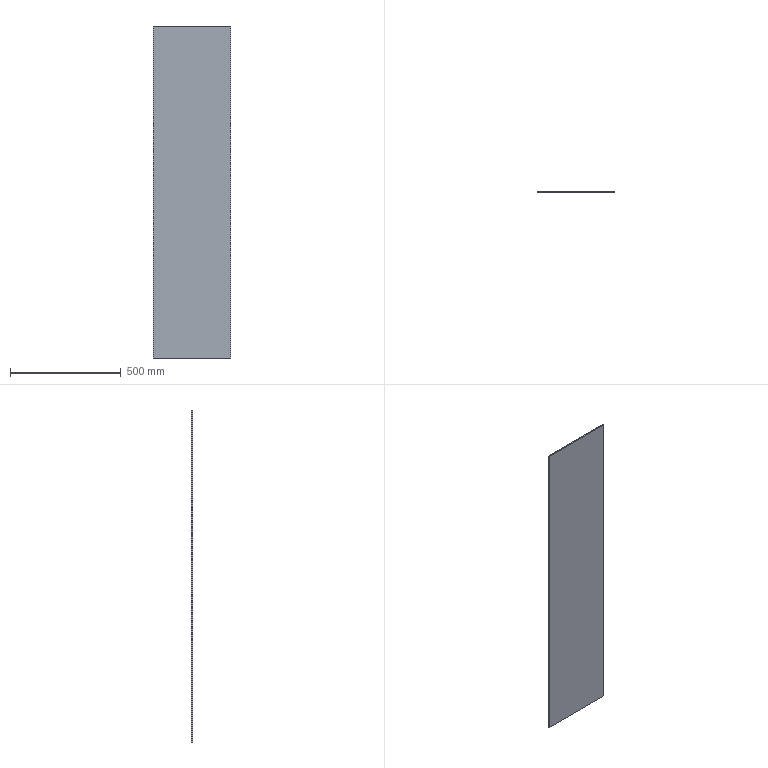Part | STEP file | Plate 2 | 1 solid | 6 faces | box 350 x 5 x 1500 mm | volume 2625000 mm3 | plane 6
STEP:
#1=CARTESIAN_POINT('',(175.,0.,750.));
#2=VERTEX_POINT('',#1);
#3=CARTESIAN_POINT('',(175.,0.,-750.));
#4=VERTEX_POINT('',#3);
#5=CARTESIAN_POINT('',(175.,0.,-750.));
#6=DIRECTION('',(0.,0.,-1.));
#7=VECTOR('',#6,1000.);
#8=LINE('',#5,#7);
#9=EDGE_CURVE('',#2,#4,#8,.T.);
#10=ORIENTED_EDGE('',*,*,#9,.T.);
#11=CARTESIAN_POINT('',(175.,5.,-750.));
#12=VERTEX_POINT('',#11);
#13=CARTESIAN_POINT('',(175.,5.,-750.));
#14=DIRECTION('',(0.,-1.,0.));
#15=VECTOR('',#14,1000.);
#16=LINE('',#13,#15);
#17=EDGE_CURVE('',#12,#4,#16,.T.);
#18=ORIENTED_EDGE('',*,*,#17,.F.);
#19=CARTESIAN_POINT('',(175.,5.,750.));
#20=VERTEX_POINT('',#19);
#21=CARTESIAN_POINT('',(175.,5.,-750.));
#22=DIRECTION('',(0.,0.,-1.));
#23=VECTOR('',#22,1000.);
#24=LINE('',#21,#23);
#25=EDGE_CURVE('',#20,#12,#24,.T.);
#26=ORIENTED_EDGE('',*,*,#25,.F.);
#27=CARTESIAN_POINT('',(175.,5.,750.));
#28=DIRECTION('',(0.,-1.,0.));
#29=VECTOR('',#28,1000.);
#30=LINE('',#27,#29);
#31=EDGE_CURVE('',#20,#2,#30,.T.);
#32=ORIENTED_EDGE('',*,*,#31,.T.);
#33=EDGE_LOOP('',(#10,#18,#26,#32));
#34=FACE_OUTER_BOUND('',#33,.T.);
#35=CARTESIAN_POINT('',(175.,5.,-750.));
#36=DIRECTION('',(-1.,0.,0.));
#37=DIRECTION('',(0.,0.,1.));
#38=AXIS2_PLACEMENT_3D('',#35,#36,#37);
#39=PLANE('',#38);
#40=ADVANCED_FACE('',(#34),#39,.F.);
#41=CARTESIAN_POINT('',(-175.,0.,-750.));
#42=VERTEX_POINT('',#41);
#43=CARTESIAN_POINT('',(-175.,0.,-750.));
#44=DIRECTION('',(-1.,0.,0.));
#45=VECTOR('',#44,1000.);
#46=LINE('',#43,#45);
#47=EDGE_CURVE('',#4,#42,#46,.T.);
#48=ORIENTED_EDGE('',*,*,#47,.T.);
#49=CARTESIAN_POINT('',(-175.,5.,-750.));
#50=VERTEX_POINT('',#49);
#51=CARTESIAN_POINT('',(-175.,5.,-750.));
#52=DIRECTION('',(0.,-1.,0.));
#53=VECTOR('',#52,1000.);
#54=LINE('',#51,#53);
#55=EDGE_CURVE('',#50,#42,#54,.T.);
#56=ORIENTED_EDGE('',*,*,#55,.F.);
#57=CARTESIAN_POINT('',(-175.,5.,-750.));
#58=DIRECTION('',(-1.,0.,0.));
#59=VECTOR('',#58,1000.);
#60=LINE('',#57,#59);
#61=EDGE_CURVE('',#12,#50,#60,.T.);
#62=ORIENTED_EDGE('',*,*,#61,.F.);
#63=ORIENTED_EDGE('',*,*,#17,.T.);
#64=EDGE_LOOP('',(#48,#56,#62,#63));
#65=FACE_OUTER_BOUND('',#64,.T.);
#66=CARTESIAN_POINT('',(-175.,5.,-750.));
#67=DIRECTION('',(0.,0.,1.));
#68=DIRECTION('',(1.,0.,0.));
#69=AXIS2_PLACEMENT_3D('',#66,#67,#68);
#70=PLANE('',#69);
#71=ADVANCED_FACE('',(#65),#70,.F.);
#72=CARTESIAN_POINT('',(-175.,0.,750.));
#73=VERTEX_POINT('',#72);
#74=CARTESIAN_POINT('',(-175.,0.,-750.));
#75=DIRECTION('',(0.,0.,1.));
#76=VECTOR('',#75,1000.);
#77=LINE('',#74,#76);
#78=EDGE_CURVE('',#42,#73,#77,.T.);
#79=ORIENTED_EDGE('',*,*,#78,.T.);
#80=CARTESIAN_POINT('',(-175.,5.,750.));
#81=VERTEX_POINT('',#80);
#82=CARTESIAN_POINT('',(-175.,5.,750.));
#83=DIRECTION('',(0.,-1.,0.));
#84=VECTOR('',#83,1000.);
#85=LINE('',#82,#84);
#86=EDGE_CURVE('',#81,#73,#85,.T.);
#87=ORIENTED_EDGE('',*,*,#86,.F.);
#88=CARTESIAN_POINT('',(-175.,5.,-750.));
#89=DIRECTION('',(0.,0.,1.));
#90=VECTOR('',#89,1000.);
#91=LINE('',#88,#90);
#92=EDGE_CURVE('',#50,#81,#91,.T.);
#93=ORIENTED_EDGE('',*,*,#92,.F.);
#94=ORIENTED_EDGE('',*,*,#55,.T.);
#95=EDGE_LOOP('',(#79,#87,#93,#94));
#96=FACE_OUTER_BOUND('',#95,.T.);
#97=CARTESIAN_POINT('',(-175.,5.,-750.));
#98=DIRECTION('',(1.,0.,0.));
#99=DIRECTION('',(0.,0.,-1.));
#100=AXIS2_PLACEMENT_3D('',#97,#98,#99);
#101=PLANE('',#100);
#102=ADVANCED_FACE('',(#96),#101,.F.);
#103=CARTESIAN_POINT('',(-175.,0.,750.));
#104=DIRECTION('',(1.,0.,0.));
#105=VECTOR('',#104,1000.);
#106=LINE('',#103,#105);
#107=EDGE_CURVE('',#73,#2,#106,.T.);
#108=ORIENTED_EDGE('',*,*,#107,.T.);
#109=ORIENTED_EDGE('',*,*,#31,.F.);
#110=CARTESIAN_POINT('',(-175.,5.,750.));
#111=DIRECTION('',(1.,0.,0.));
#112=VECTOR('',#111,1000.);
#113=LINE('',#110,#112);
#114=EDGE_CURVE('',#81,#20,#113,.T.);
#115=ORIENTED_EDGE('',*,*,#114,.F.);
#116=ORIENTED_EDGE('',*,*,#86,.T.);
#117=EDGE_LOOP('',(#108,#109,#115,#116));
#118=FACE_OUTER_BOUND('',#117,.T.);
#119=CARTESIAN_POINT('',(-175.,5.,750.));
#120=DIRECTION('',(0.,0.,-1.));
#121=DIRECTION('',(-1.,0.,0.));
#122=AXIS2_PLACEMENT_3D('',#119,#120,#121);
#123=PLANE('',#122);
#124=ADVANCED_FACE('',(#118),#123,.F.);
#125=ORIENTED_EDGE('',*,*,#25,.T.);
#126=ORIENTED_EDGE('',*,*,#61,.T.);
#127=ORIENTED_EDGE('',*,*,#92,.T.);
#128=ORIENTED_EDGE('',*,*,#114,.T.);
#129=EDGE_LOOP('',(#125,#126,#127,#128));
#130=FACE_OUTER_BOUND('',#129,.T.);
#131=CARTESIAN_POINT('',(0.,5.,0.));
#132=DIRECTION('',(0.,1.,0.));
#133=DIRECTION('',(0.,0.,1.));
#134=AXIS2_PLACEMENT_3D('',#131,#132,#133);
#135=PLANE('',#134);
#136=ADVANCED_FACE('',(#130),#135,.T.);
#137=ORIENTED_EDGE('',*,*,#9,.F.);
#138=ORIENTED_EDGE('',*,*,#107,.F.);
#139=ORIENTED_EDGE('',*,*,#78,.F.);
#140=ORIENTED_EDGE('',*,*,#47,.F.);
#141=EDGE_LOOP('',(#137,#138,#139,#140));
#142=FACE_OUTER_BOUND('',#141,.T.);
#143=CARTESIAN_POINT('',(0.,0.,0.));
#144=DIRECTION('',(0.,1.,0.));
#145=DIRECTION('',(0.,0.,1.));
#146=AXIS2_PLACEMENT_3D('',#143,#144,#145);
#147=PLANE('',#146);
#148=ADVANCED_FACE('',(#142),#147,.F.);
#149=CLOSED_SHELL('',(#40,#71,#102,#124,#136,#148));
#150=MANIFOLD_SOLID_BREP('',#149);
#151=CARTESIAN_POINT('',(0.,0.,0.));
#152=DIRECTION('',(0.,0.,1.));
#153=DIRECTION('',(1.,0.,0.));
#154=AXIS2_PLACEMENT_3D('',#151,#152,#153);
#155=(LENGTH_UNIT()NAMED_UNIT(*)SI_UNIT(.MILLI.,.METRE.));
#156=UNCERTAINTY_MEASURE_WITH_UNIT(LENGTH_MEASURE(0.00001),#155,'','');
#157=(NAMED_UNIT(*)PLANE_ANGLE_UNIT()SI_UNIT($,.RADIAN.));
#158=(NAMED_UNIT(*)SI_UNIT($,.STERADIAN.)SOLID_ANGLE_UNIT());
#159=(GEOMETRIC_REPRESENTATION_CONTEXT(3)GLOBAL_UNCERTAINTY_ASSIGNED_CONTEXT((#156))GLOBAL_UNIT_ASSIGNED_CONTEXT((#155,#157,#158))REPRESENTATION_CONTEXT('',''));
#160=ADVANCED_BREP_SHAPE_REPRESENTATION('',(#150,#154),#159);